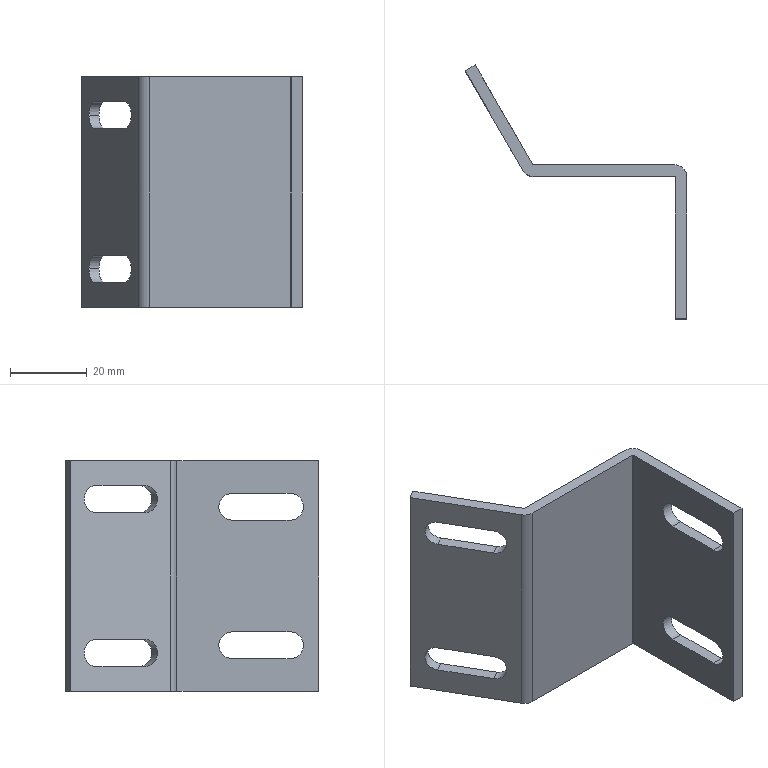Part | STEP file | Z Travel Bracket | 1 solid | 32 faces | box 57.598 x 65.981 x 60 mm | volume 17695 mm3 | plane 18 | cylinder 14 | commonest cylinder face diameters 7 x10 0.2 x2 6.2 x2
STEP:
#1=CARTESIAN_POINT('',(88.934,74.807,53.5));
#2=VERTEX_POINT('',#1);
#3=CARTESIAN_POINT('',(87.184,77.838,50.));
#4=VERTEX_POINT('',#3);
#5=CARTESIAN_POINT('',(88.934,74.807,50.));
#6=DIRECTION('',(-0.866,-0.5,0.));
#7=DIRECTION('',(-0.5,0.866,0.));
#8=AXIS2_PLACEMENT_3D('',#5,#6,#7);
#9=CIRCLE('',#8,3.5);
#10=EDGE_CURVE('',#2,#4,#9,.T.);
#11=ORIENTED_EDGE('',*,*,#10,.T.);
#12=CARTESIAN_POINT('',(89.782,79.338,50.));
#13=VERTEX_POINT('',#12);
#14=CARTESIAN_POINT('',(81.122,74.338,50.));
#15=DIRECTION('',(0.866,0.5,0.));
#16=VECTOR('',#15,1000.);
#17=LINE('',#14,#16);
#18=EDGE_CURVE('',#4,#13,#17,.T.);
#19=ORIENTED_EDGE('',*,*,#18,.T.);
#20=CARTESIAN_POINT('',(91.532,76.307,53.5));
#21=VERTEX_POINT('',#20);
#22=CARTESIAN_POINT('',(91.532,76.307,50.));
#23=DIRECTION('',(-0.866,-0.5,0.));
#24=DIRECTION('',(-0.5,0.866,0.));
#25=AXIS2_PLACEMENT_3D('',#22,#23,#24);
#26=CIRCLE('',#25,3.5);
#27=EDGE_CURVE('',#21,#13,#26,.T.);
#28=ORIENTED_EDGE('',*,*,#27,.F.);
#29=CARTESIAN_POINT('',(82.872,71.307,53.5));
#30=DIRECTION('',(0.866,0.5,0.));
#31=VECTOR('',#30,1000.);
#32=LINE('',#29,#31);
#33=EDGE_CURVE('',#2,#21,#32,.T.);
#34=ORIENTED_EDGE('',*,*,#33,.F.);
#35=EDGE_LOOP('',(#11,#19,#28,#34));
#36=FACE_OUTER_BOUND('',#35,.T.);
#37=CARTESIAN_POINT('',(82.872,71.307,50.));
#38=DIRECTION('',(0.866,0.5,0.));
#39=DIRECTION('',(-0.5,0.866,0.));
#40=AXIS2_PLACEMENT_3D('',#37,#38,#39);
#41=CYLINDRICAL_SURFACE('',#40,3.5);
#42=ADVANCED_FACE('',(#36),#41,.F.);
#43=CARTESIAN_POINT('',(88.934,74.807,13.5));
#44=VERTEX_POINT('',#43);
#45=CARTESIAN_POINT('',(87.184,77.838,10.));
#46=VERTEX_POINT('',#45);
#47=CARTESIAN_POINT('',(88.934,74.807,10.));
#48=DIRECTION('',(-0.866,-0.5,0.));
#49=DIRECTION('',(-0.5,0.866,0.));
#50=AXIS2_PLACEMENT_3D('',#47,#48,#49);
#51=CIRCLE('',#50,3.5);
#52=EDGE_CURVE('',#44,#46,#51,.T.);
#53=ORIENTED_EDGE('',*,*,#52,.T.);
#54=CARTESIAN_POINT('',(89.782,79.338,10.));
#55=VERTEX_POINT('',#54);
#56=CARTESIAN_POINT('',(81.122,74.338,10.));
#57=DIRECTION('',(0.866,0.5,0.));
#58=VECTOR('',#57,1000.);
#59=LINE('',#56,#58);
#60=EDGE_CURVE('',#46,#55,#59,.T.);
#61=ORIENTED_EDGE('',*,*,#60,.T.);
#62=CARTESIAN_POINT('',(91.532,76.307,13.5));
#63=VERTEX_POINT('',#62);
#64=CARTESIAN_POINT('',(91.532,76.307,10.));
#65=DIRECTION('',(-0.866,-0.5,0.));
#66=DIRECTION('',(-0.5,0.866,0.));
#67=AXIS2_PLACEMENT_3D('',#64,#65,#66);
#68=CIRCLE('',#67,3.5);
#69=EDGE_CURVE('',#63,#55,#68,.T.);
#70=ORIENTED_EDGE('',*,*,#69,.F.);
#71=CARTESIAN_POINT('',(82.872,71.307,13.5));
#72=DIRECTION('',(0.866,0.5,0.));
#73=VECTOR('',#72,1000.);
#74=LINE('',#71,#73);
#75=EDGE_CURVE('',#44,#63,#74,.T.);
#76=ORIENTED_EDGE('',*,*,#75,.F.);
#77=EDGE_LOOP('',(#53,#61,#70,#76));
#78=FACE_OUTER_BOUND('',#77,.T.);
#79=CARTESIAN_POINT('',(82.872,71.307,10.));
#80=DIRECTION('',(0.866,0.5,0.));
#81=DIRECTION('',(-0.5,0.866,0.));
#82=AXIS2_PLACEMENT_3D('',#79,#80,#81);
#83=CYLINDRICAL_SURFACE('',#82,3.5);
#84=ADVANCED_FACE('',(#78),#83,.F.);
#85=CARTESIAN_POINT('',(139.682,53.821,60.));
#86=VERTEX_POINT('',#85);
#87=CARTESIAN_POINT('',(139.682,53.821,0.));
#88=VERTEX_POINT('',#87);
#89=CARTESIAN_POINT('',(139.682,53.821,60.));
#90=DIRECTION('',(0.,0.,-1.));
#91=VECTOR('',#90,1000.);
#92=LINE('',#89,#91);
#93=EDGE_CURVE('',#86,#88,#92,.T.);
#94=ORIENTED_EDGE('',*,*,#93,.F.);
#95=CARTESIAN_POINT('',(102.84,53.821,60.));
#96=VERTEX_POINT('',#95);
#97=CARTESIAN_POINT('',(102.782,53.821,60.));
#98=DIRECTION('',(1.,0.,0.));
#99=VECTOR('',#98,1000.);
#100=LINE('',#97,#99);
#101=EDGE_CURVE('',#96,#86,#100,.T.);
#102=ORIENTED_EDGE('',*,*,#101,.F.);
#103=CARTESIAN_POINT('',(102.84,53.821,0.));
#104=VERTEX_POINT('',#103);
#105=CARTESIAN_POINT('',(102.84,53.821,60.));
#106=DIRECTION('',(0.,0.,1.));
#107=VECTOR('',#106,1000.);
#108=LINE('',#105,#107);
#109=EDGE_CURVE('',#104,#96,#108,.T.);
#110=ORIENTED_EDGE('',*,*,#109,.F.);
#111=CARTESIAN_POINT('',(102.782,53.821,0.));
#112=DIRECTION('',(-1.,0.,0.));
#113=VECTOR('',#112,1000.);
#114=LINE('',#111,#113);
#115=EDGE_CURVE('',#88,#104,#114,.T.);
#116=ORIENTED_EDGE('',*,*,#115,.F.);
#117=EDGE_LOOP('',(#94,#102,#110,#116));
#118=FACE_OUTER_BOUND('',#117,.T.);
#119=CARTESIAN_POINT('',(102.782,53.821,60.));
#120=DIRECTION('',(0.,1.,0.));
#121=DIRECTION('',(0.,0.,1.));
#122=AXIS2_PLACEMENT_3D('',#119,#120,#121);
#123=PLANE('',#122);
#124=ADVANCED_FACE('',(#118),#123,.F.);
#125=ORIENTED_EDGE('',*,*,#115,.T.);
#126=CARTESIAN_POINT('',(100.155,55.371,0.));
#127=VERTEX_POINT('',#126);
#128=CARTESIAN_POINT('',(102.84,56.921,0.));
#129=DIRECTION('',(0.,0.,1.));
#130=DIRECTION('',(-1.,0.,0.));
#131=AXIS2_PLACEMENT_3D('',#128,#129,#130);
#132=CIRCLE('',#131,3.1);
#133=EDGE_CURVE('',#127,#104,#132,.T.);
#134=ORIENTED_EDGE('',*,*,#133,.F.);
#135=CARTESIAN_POINT('',(85.184,81.302,0.));
#136=VERTEX_POINT('',#135);
#137=CARTESIAN_POINT('',(85.184,81.302,0.));
#138=DIRECTION('',(-0.5,0.866,0.));
#139=VECTOR('',#138,1000.);
#140=LINE('',#137,#139);
#141=EDGE_CURVE('',#127,#136,#140,.T.);
#142=ORIENTED_EDGE('',*,*,#141,.T.);
#143=CARTESIAN_POINT('',(87.782,82.802,0.));
#144=VERTEX_POINT('',#143);
#145=CARTESIAN_POINT('',(85.184,81.302,0.));
#146=DIRECTION('',(0.866,0.5,0.));
#147=VECTOR('',#146,1000.);
#148=LINE('',#145,#147);
#149=EDGE_CURVE('',#136,#144,#148,.T.);
#150=ORIENTED_EDGE('',*,*,#149,.T.);
#151=CARTESIAN_POINT('',(102.753,56.871,0.));
#152=VERTEX_POINT('',#151);
#153=CARTESIAN_POINT('',(87.782,82.802,0.));
#154=DIRECTION('',(0.5,-0.866,0.));
#155=VECTOR('',#154,1000.);
#156=LINE('',#153,#155);
#157=EDGE_CURVE('',#144,#152,#156,.T.);
#158=ORIENTED_EDGE('',*,*,#157,.T.);
#159=CARTESIAN_POINT('',(102.84,56.821,0.));
#160=VERTEX_POINT('',#159);
#161=CARTESIAN_POINT('',(102.84,56.921,0.));
#162=DIRECTION('',(0.,0.,1.));
#163=DIRECTION('',(-1.,0.,0.));
#164=AXIS2_PLACEMENT_3D('',#161,#162,#163);
#165=CIRCLE('',#164,0.1);
#166=EDGE_CURVE('',#152,#160,#165,.T.);
#167=ORIENTED_EDGE('',*,*,#166,.T.);
#168=CARTESIAN_POINT('',(139.682,56.821,0.));
#169=VERTEX_POINT('',#168);
#170=CARTESIAN_POINT('',(139.782,56.821,0.));
#171=DIRECTION('',(1.,0.,0.));
#172=VECTOR('',#171,1000.);
#173=LINE('',#170,#172);
#174=EDGE_CURVE('',#160,#169,#173,.T.);
#175=ORIENTED_EDGE('',*,*,#174,.T.);
#176=CARTESIAN_POINT('',(142.782,53.721,0.));
#177=VERTEX_POINT('',#176);
#178=CARTESIAN_POINT('',(139.682,53.721,0.));
#179=DIRECTION('',(0.,0.,-1.));
#180=DIRECTION('',(-1.,0.,0.));
#181=AXIS2_PLACEMENT_3D('',#178,#179,#180);
#182=CIRCLE('',#181,3.1);
#183=EDGE_CURVE('',#169,#177,#182,.T.);
#184=ORIENTED_EDGE('',*,*,#183,.T.);
#185=CARTESIAN_POINT('',(142.782,16.821,0.));
#186=VERTEX_POINT('',#185);
#187=CARTESIAN_POINT('',(142.782,53.721,0.));
#188=DIRECTION('',(0.,1.,0.));
#189=VECTOR('',#188,1000.);
#190=LINE('',#187,#189);
#191=EDGE_CURVE('',#186,#177,#190,.T.);
#192=ORIENTED_EDGE('',*,*,#191,.F.);
#193=CARTESIAN_POINT('',(139.782,16.821,0.));
#194=VERTEX_POINT('',#193);
#195=CARTESIAN_POINT('',(139.682,16.821,0.));
#196=DIRECTION('',(1.,0.,0.));
#197=VECTOR('',#196,1000.);
#198=LINE('',#195,#197);
#199=EDGE_CURVE('',#194,#186,#198,.T.);
#200=ORIENTED_EDGE('',*,*,#199,.F.);
#201=CARTESIAN_POINT('',(139.782,53.721,0.));
#202=VERTEX_POINT('',#201);
#203=CARTESIAN_POINT('',(139.782,56.821,0.));
#204=DIRECTION('',(0.,1.,0.));
#205=VECTOR('',#204,1000.);
#206=LINE('',#203,#205);
#207=EDGE_CURVE('',#194,#202,#206,.T.);
#208=ORIENTED_EDGE('',*,*,#207,.T.);
#209=CARTESIAN_POINT('',(139.682,53.721,0.));
#210=DIRECTION('',(0.,0.,1.));
#211=DIRECTION('',(-1.,0.,0.));
#212=AXIS2_PLACEMENT_3D('',#209,#210,#211);
#213=CIRCLE('',#212,0.1);
#214=EDGE_CURVE('',#202,#88,#213,.T.);
#215=ORIENTED_EDGE('',*,*,#214,.T.);
#216=EDGE_LOOP('',(#125,#134,#142,#150,#158,#167,#175,#184,#192,#200,#208,#215));
#217=FACE_OUTER_BOUND('',#216,.T.);
#218=CARTESIAN_POINT('',(139.782,53.721,0.));
#219=DIRECTION('',(0.,0.,-1.));
#220=DIRECTION('',(-1.,0.,0.));
#221=AXIS2_PLACEMENT_3D('',#218,#219,#220);
#222=PLANE('',#221);
#223=ADVANCED_FACE('',(#217),#222,.T.);
#224=CARTESIAN_POINT('',(139.782,53.721,60.));
#225=VERTEX_POINT('',#224);
#226=CARTESIAN_POINT('',(139.782,53.721,60.));
#227=DIRECTION('',(0.,0.,-1.));
#228=VECTOR('',#227,1000.);
#229=LINE('',#226,#228);
#230=EDGE_CURVE('',#225,#202,#229,.T.);
#231=ORIENTED_EDGE('',*,*,#230,.F.);
#232=CARTESIAN_POINT('',(139.682,53.721,60.));
#233=DIRECTION('',(0.,0.,-1.));
#234=DIRECTION('',(-1.,0.,0.));
#235=AXIS2_PLACEMENT_3D('',#232,#233,#234);
#236=CIRCLE('',#235,0.1);
#237=EDGE_CURVE('',#86,#225,#236,.T.);
#238=ORIENTED_EDGE('',*,*,#237,.F.);
#239=ORIENTED_EDGE('',*,*,#93,.T.);
#240=ORIENTED_EDGE('',*,*,#214,.F.);
#241=EDGE_LOOP('',(#231,#238,#239,#240));
#242=FACE_OUTER_BOUND('',#241,.T.);
#243=CARTESIAN_POINT('',(139.682,53.721,60.));
#244=DIRECTION('',(0.,0.,-1.));
#245=DIRECTION('',(-1.,0.,0.));
#246=AXIS2_PLACEMENT_3D('',#243,#244,#245);
#247=CYLINDRICAL_SURFACE('',#246,0.1);
#248=ADVANCED_FACE('',(#242),#247,.F.);
#249=ORIENTED_EDGE('',*,*,#101,.T.);
#250=ORIENTED_EDGE('',*,*,#237,.T.);
#251=CARTESIAN_POINT('',(139.782,16.821,60.));
#252=VERTEX_POINT('',#251);
#253=CARTESIAN_POINT('',(139.782,56.821,60.));
#254=DIRECTION('',(0.,-1.,0.));
#255=VECTOR('',#254,1000.);
#256=LINE('',#253,#255);
#257=EDGE_CURVE('',#225,#252,#256,.T.);
#258=ORIENTED_EDGE('',*,*,#257,.T.);
#259=CARTESIAN_POINT('',(142.782,16.821,60.));
#260=VERTEX_POINT('',#259);
#261=CARTESIAN_POINT('',(142.782,16.821,60.));
#262=DIRECTION('',(-1.,0.,0.));
#263=VECTOR('',#262,1000.);
#264=LINE('',#261,#263);
#265=EDGE_CURVE('',#260,#252,#264,.T.);
#266=ORIENTED_EDGE('',*,*,#265,.F.);
#267=CARTESIAN_POINT('',(142.782,53.721,60.));
#268=VERTEX_POINT('',#267);
#269=CARTESIAN_POINT('',(142.782,53.821,60.));
#270=DIRECTION('',(0.,1.,0.));
#271=VECTOR('',#270,1000.);
#272=LINE('',#269,#271);
#273=EDGE_CURVE('',#260,#268,#272,.T.);
#274=ORIENTED_EDGE('',*,*,#273,.T.);
#275=CARTESIAN_POINT('',(139.682,56.821,60.));
#276=VERTEX_POINT('',#275);
#277=CARTESIAN_POINT('',(139.682,53.721,60.));
#278=DIRECTION('',(0.,0.,1.));
#279=DIRECTION('',(-1.,0.,0.));
#280=AXIS2_PLACEMENT_3D('',#277,#278,#279);
#281=CIRCLE('',#280,3.1);
#282=EDGE_CURVE('',#268,#276,#281,.T.);
#283=ORIENTED_EDGE('',*,*,#282,.T.);
#284=CARTESIAN_POINT('',(102.84,56.821,60.));
#285=VERTEX_POINT('',#284);
#286=CARTESIAN_POINT('',(100.155,56.821,60.));
#287=DIRECTION('',(-1.,0.,0.));
#288=VECTOR('',#287,1000.);
#289=LINE('',#286,#288);
#290=EDGE_CURVE('',#276,#285,#289,.T.);
#291=ORIENTED_EDGE('',*,*,#290,.T.);
#292=CARTESIAN_POINT('',(102.753,56.871,60.));
#293=VERTEX_POINT('',#292);
#294=CARTESIAN_POINT('',(102.84,56.921,60.));
#295=DIRECTION('',(0.,0.,-1.));
#296=DIRECTION('',(-1.,0.,0.));
#297=AXIS2_PLACEMENT_3D('',#294,#295,#296);
#298=CIRCLE('',#297,0.1);
#299=EDGE_CURVE('',#285,#293,#298,.T.);
#300=ORIENTED_EDGE('',*,*,#299,.T.);
#301=CARTESIAN_POINT('',(87.782,82.802,60.));
#302=VERTEX_POINT('',#301);
#303=CARTESIAN_POINT('',(102.753,56.871,60.));
#304=DIRECTION('',(-0.5,0.866,0.));
#305=VECTOR('',#304,1000.);
#306=LINE('',#303,#305);
#307=EDGE_CURVE('',#293,#302,#306,.T.);
#308=ORIENTED_EDGE('',*,*,#307,.T.);
#309=CARTESIAN_POINT('',(85.184,81.302,60.));
#310=VERTEX_POINT('',#309);
#311=CARTESIAN_POINT('',(87.782,82.802,60.));
#312=DIRECTION('',(-0.866,-0.5,0.));
#313=VECTOR('',#312,1000.);
#314=LINE('',#311,#313);
#315=EDGE_CURVE('',#302,#310,#314,.T.);
#316=ORIENTED_EDGE('',*,*,#315,.T.);
#317=CARTESIAN_POINT('',(100.155,55.371,60.));
#318=VERTEX_POINT('',#317);
#319=CARTESIAN_POINT('',(85.184,81.302,60.));
#320=DIRECTION('',(0.5,-0.866,0.));
#321=VECTOR('',#320,1000.);
#322=LINE('',#319,#321);
#323=EDGE_CURVE('',#310,#318,#322,.T.);
#324=ORIENTED_EDGE('',*,*,#323,.T.);
#325=CARTESIAN_POINT('',(102.84,56.921,60.));
#326=DIRECTION('',(0.,0.,-1.));
#327=DIRECTION('',(-1.,0.,0.));
#328=AXIS2_PLACEMENT_3D('',#325,#326,#327);
#329=CIRCLE('',#328,3.1);
#330=EDGE_CURVE('',#96,#318,#329,.T.);
#331=ORIENTED_EDGE('',*,*,#330,.F.);
#332=EDGE_LOOP('',(#249,#250,#258,#266,#274,#283,#291,#300,#308,#316,#324,#331));
#333=FACE_OUTER_BOUND('',#332,.T.);
#334=CARTESIAN_POINT('',(100.155,55.371,60.));
#335=DIRECTION('',(0.,0.,1.));
#336=DIRECTION('',(1.,0.,0.));
#337=AXIS2_PLACEMENT_3D('',#334,#335,#336);
#338=PLANE('',#337);
#339=ADVANCED_FACE('',(#333),#338,.T.);
#340=ORIENTED_EDGE('',*,*,#330,.T.);
#341=CARTESIAN_POINT('',(100.155,55.371,60.));
#342=DIRECTION('',(0.,0.,-1.));
#343=VECTOR('',#342,1000.);
#344=LINE('',#341,#343);
#345=EDGE_CURVE('',#318,#127,#344,.T.);
#346=ORIENTED_EDGE('',*,*,#345,.T.);
#347=ORIENTED_EDGE('',*,*,#133,.T.);
#348=ORIENTED_EDGE('',*,*,#109,.T.);
#349=EDGE_LOOP('',(#340,#346,#347,#348));
#350=FACE_OUTER_BOUND('',#349,.T.);
#351=CARTESIAN_POINT('',(102.84,56.921,60.));
#352=DIRECTION('',(0.,0.,-1.));
#353=DIRECTION('',(-1.,0.,0.));
#354=AXIS2_PLACEMENT_3D('',#351,#352,#353);
#355=CYLINDRICAL_SURFACE('',#354,3.1);
#356=ADVANCED_FACE('',(#350),#355,.T.);
#357=ORIENTED_EDGE('',*,*,#290,.F.);
#358=CARTESIAN_POINT('',(139.682,56.821,60.));
#359=DIRECTION('',(0.,0.,-1.));
#360=VECTOR('',#359,1000.);
#361=LINE('',#358,#360);
#362=EDGE_CURVE('',#276,#169,#361,.T.);
#363=ORIENTED_EDGE('',*,*,#362,.T.);
#364=ORIENTED_EDGE('',*,*,#174,.F.);
#365=CARTESIAN_POINT('',(102.84,56.821,60.));
#366=DIRECTION('',(0.,0.,1.));
#367=VECTOR('',#366,1000.);
#368=LINE('',#365,#367);
#369=EDGE_CURVE('',#160,#285,#368,.T.);
#370=ORIENTED_EDGE('',*,*,#369,.T.);
#371=EDGE_LOOP('',(#357,#363,#364,#370));
#372=FACE_OUTER_BOUND('',#371,.T.);
#373=CARTESIAN_POINT('',(102.782,56.821,60.));
#374=DIRECTION('',(0.,1.,0.));
#375=DIRECTION('',(0.,0.,1.));
#376=AXIS2_PLACEMENT_3D('',#373,#374,#375);
#377=PLANE('',#376);
#378=ADVANCED_FACE('',(#372),#377,.T.);
#379=CARTESIAN_POINT('',(139.782,16.821,60.));
#380=DIRECTION('',(0.,0.,-1.));
#381=VECTOR('',#380,1000.);
#382=LINE('',#379,#381);
#383=EDGE_CURVE('',#252,#194,#382,.T.);
#384=ORIENTED_EDGE('',*,*,#383,.F.);
#385=ORIENTED_EDGE('',*,*,#257,.F.);
#386=ORIENTED_EDGE('',*,*,#230,.T.);
#387=ORIENTED_EDGE('',*,*,#207,.F.);
#388=EDGE_LOOP('',(#384,#385,#386,#387));
#389=FACE_OUTER_BOUND('',#388,.T.);
#390=CARTESIAN_POINT('',(139.782,39.321,51.5));
#391=VERTEX_POINT('',#390);
#392=CARTESIAN_POINT('',(139.782,39.321,44.5));
#393=VERTEX_POINT('',#392);
#394=CARTESIAN_POINT('',(139.782,39.321,48.));
#395=DIRECTION('',(-1.,0.,0.));
#396=DIRECTION('',(0.,0.,-1.));
#397=AXIS2_PLACEMENT_3D('',#394,#395,#396);
#398=CIRCLE('',#397,3.5);
#399=EDGE_CURVE('',#391,#393,#398,.T.);
#400=ORIENTED_EDGE('',*,*,#399,.F.);
#401=CARTESIAN_POINT('',(139.782,24.321,51.5));
#402=VERTEX_POINT('',#401);
#403=CARTESIAN_POINT('',(139.782,56.821,51.5));
#404=DIRECTION('',(0.,1.,0.));
#405=VECTOR('',#404,1000.);
#406=LINE('',#403,#405);
#407=EDGE_CURVE('',#402,#391,#406,.T.);
#408=ORIENTED_EDGE('',*,*,#407,.F.);
#409=CARTESIAN_POINT('',(139.782,24.321,44.5));
#410=VERTEX_POINT('',#409);
#411=CARTESIAN_POINT('',(139.782,24.321,48.));
#412=DIRECTION('',(-1.,0.,0.));
#413=DIRECTION('',(0.,0.,-1.));
#414=AXIS2_PLACEMENT_3D('',#411,#412,#413);
#415=CIRCLE('',#414,3.5);
#416=EDGE_CURVE('',#410,#402,#415,.T.);
#417=ORIENTED_EDGE('',*,*,#416,.F.);
#418=CARTESIAN_POINT('',(139.782,56.821,44.5));
#419=DIRECTION('',(0.,-1.,0.));
#420=VECTOR('',#419,1000.);
#421=LINE('',#418,#420);
#422=EDGE_CURVE('',#393,#410,#421,.T.);
#423=ORIENTED_EDGE('',*,*,#422,.F.);
#424=EDGE_LOOP('',(#400,#408,#417,#423));
#425=FACE_BOUND('',#424,.T.);
#426=CARTESIAN_POINT('',(139.782,39.321,15.5));
#427=VERTEX_POINT('',#426);
#428=CARTESIAN_POINT('',(139.782,39.321,8.5));
#429=VERTEX_POINT('',#428);
#430=CARTESIAN_POINT('',(139.782,39.321,12.));
#431=DIRECTION('',(-1.,0.,0.));
#432=DIRECTION('',(0.,0.,-1.));
#433=AXIS2_PLACEMENT_3D('',#430,#431,#432);
#434=CIRCLE('',#433,3.5);
#435=EDGE_CURVE('',#427,#429,#434,.T.);
#436=ORIENTED_EDGE('',*,*,#435,.F.);
#437=CARTESIAN_POINT('',(139.782,24.321,15.5));
#438=VERTEX_POINT('',#437);
#439=CARTESIAN_POINT('',(139.782,56.821,15.5));
#440=DIRECTION('',(0.,1.,0.));
#441=VECTOR('',#440,1000.);
#442=LINE('',#439,#441);
#443=EDGE_CURVE('',#438,#427,#442,.T.);
#444=ORIENTED_EDGE('',*,*,#443,.F.);
#445=CARTESIAN_POINT('',(139.782,24.321,8.5));
#446=VERTEX_POINT('',#445);
#447=CARTESIAN_POINT('',(139.782,24.321,12.));
#448=DIRECTION('',(-1.,0.,0.));
#449=DIRECTION('',(0.,0.,-1.));
#450=AXIS2_PLACEMENT_3D('',#447,#448,#449);
#451=CIRCLE('',#450,3.5);
#452=EDGE_CURVE('',#446,#438,#451,.T.);
#453=ORIENTED_EDGE('',*,*,#452,.F.);
#454=CARTESIAN_POINT('',(139.782,56.821,8.5));
#455=DIRECTION('',(0.,-1.,0.));
#456=VECTOR('',#455,1000.);
#457=LINE('',#454,#456);
#458=EDGE_CURVE('',#429,#446,#457,.T.);
#459=ORIENTED_EDGE('',*,*,#458,.F.);
#460=EDGE_LOOP('',(#436,#444,#453,#459));
#461=FACE_BOUND('',#460,.T.);
#462=CARTESIAN_POINT('',(139.782,56.821,60.));
#463=DIRECTION('',(1.,0.,0.));
#464=DIRECTION('',(0.,0.,-1.));
#465=AXIS2_PLACEMENT_3D('',#462,#463,#464);
#466=PLANE('',#465);
#467=ADVANCED_FACE('',(#389,#425,#461),#466,.F.);
#468=ORIENTED_EDGE('',*,*,#345,.F.);
#469=ORIENTED_EDGE('',*,*,#323,.F.);
#470=CARTESIAN_POINT('',(85.184,81.302,60.));
#471=DIRECTION('',(0.,0.,1.));
#472=VECTOR('',#471,1000.);
#473=LINE('',#470,#472);
#474=EDGE_CURVE('',#136,#310,#473,.T.);
#475=ORIENTED_EDGE('',*,*,#474,.F.);
#476=ORIENTED_EDGE('',*,*,#141,.F.);
#477=EDGE_LOOP('',(#468,#469,#475,#476));
#478=FACE_OUTER_BOUND('',#477,.T.);
#479=ORIENTED_EDGE('',*,*,#10,.F.);
#480=CARTESIAN_POINT('',(96.434,61.816,53.5));
#481=VERTEX_POINT('',#480);
#482=CARTESIAN_POINT('',(85.184,81.302,53.5));
#483=DIRECTION('',(-0.5,0.866,0.));
#484=VECTOR('',#483,1000.);
#485=LINE('',#482,#484);
#486=EDGE_CURVE('',#481,#2,#485,.T.);
#487=ORIENTED_EDGE('',*,*,#486,.F.);
#488=CARTESIAN_POINT('',(96.434,61.816,46.5));
#489=VERTEX_POINT('',#488);
#490=CARTESIAN_POINT('',(96.434,61.816,50.));
#491=DIRECTION('',(-0.866,-0.5,0.));
#492=DIRECTION('',(-0.5,0.866,0.));
#493=AXIS2_PLACEMENT_3D('',#490,#491,#492);
#494=CIRCLE('',#493,3.5);
#495=EDGE_CURVE('',#489,#481,#494,.T.);
#496=ORIENTED_EDGE('',*,*,#495,.F.);
#497=CARTESIAN_POINT('',(88.934,74.807,46.5));
#498=VERTEX_POINT('',#497);
#499=CARTESIAN_POINT('',(85.184,81.302,46.5));
#500=DIRECTION('',(0.5,-0.866,0.));
#501=VECTOR('',#500,1000.);
#502=LINE('',#499,#501);
#503=EDGE_CURVE('',#498,#489,#502,.T.);
#504=ORIENTED_EDGE('',*,*,#503,.F.);
#505=CARTESIAN_POINT('',(88.934,74.807,50.));
#506=DIRECTION('',(-0.866,-0.5,0.));
#507=DIRECTION('',(-0.5,0.866,0.));
#508=AXIS2_PLACEMENT_3D('',#505,#506,#507);
#509=CIRCLE('',#508,3.5);
#510=EDGE_CURVE('',#4,#498,#509,.T.);
#511=ORIENTED_EDGE('',*,*,#510,.F.);
#512=EDGE_LOOP('',(#479,#487,#496,#504,#511));
#513=FACE_BOUND('',#512,.T.);
#514=ORIENTED_EDGE('',*,*,#52,.F.);
#515=CARTESIAN_POINT('',(96.434,61.816,13.5));
#516=VERTEX_POINT('',#515);
#517=CARTESIAN_POINT('',(85.184,81.302,13.5));
#518=DIRECTION('',(-0.5,0.866,0.));
#519=VECTOR('',#518,1000.);
#520=LINE('',#517,#519);
#521=EDGE_CURVE('',#516,#44,#520,.T.);
#522=ORIENTED_EDGE('',*,*,#521,.F.);
#523=CARTESIAN_POINT('',(96.434,61.816,6.5));
#524=VERTEX_POINT('',#523);
#525=CARTESIAN_POINT('',(96.434,61.816,10.));
#526=DIRECTION('',(-0.866,-0.5,0.));
#527=DIRECTION('',(-0.5,0.866,0.));
#528=AXIS2_PLACEMENT_3D('',#525,#526,#527);
#529=CIRCLE('',#528,3.5);
#530=EDGE_CURVE('',#524,#516,#529,.T.);
#531=ORIENTED_EDGE('',*,*,#530,.F.);
#532=CARTESIAN_POINT('',(88.934,74.807,6.5));
#533=VERTEX_POINT('',#532);
#534=CARTESIAN_POINT('',(85.184,81.302,6.5));
#535=DIRECTION('',(0.5,-0.866,0.));
#536=VECTOR('',#535,1000.);
#537=LINE('',#534,#536);
#538=EDGE_CURVE('',#533,#524,#537,.T.);
#539=ORIENTED_EDGE('',*,*,#538,.F.);
#540=CARTESIAN_POINT('',(88.934,74.807,10.));
#541=DIRECTION('',(-0.866,-0.5,0.));
#542=DIRECTION('',(-0.5,0.866,0.));
#543=AXIS2_PLACEMENT_3D('',#540,#541,#542);
#544=CIRCLE('',#543,3.5);
#545=EDGE_CURVE('',#46,#533,#544,.T.);
#546=ORIENTED_EDGE('',*,*,#545,.F.);
#547=EDGE_LOOP('',(#514,#522,#531,#539,#546));
#548=FACE_BOUND('',#547,.T.);
#549=CARTESIAN_POINT('',(85.184,81.302,60.));
#550=DIRECTION('',(0.866,0.5,0.));
#551=DIRECTION('',(-0.5,0.866,0.));
#552=AXIS2_PLACEMENT_3D('',#549,#550,#551);
#553=PLANE('',#552);
#554=ADVANCED_FACE('',(#478,#513,#548),#553,.F.);
#555=ORIENTED_EDGE('',*,*,#282,.F.);
#556=CARTESIAN_POINT('',(142.782,53.721,60.));
#557=DIRECTION('',(0.,0.,-1.));
#558=VECTOR('',#557,1000.);
#559=LINE('',#556,#558);
#560=EDGE_CURVE('',#268,#177,#559,.T.);
#561=ORIENTED_EDGE('',*,*,#560,.T.);
#562=ORIENTED_EDGE('',*,*,#183,.F.);
#563=ORIENTED_EDGE('',*,*,#362,.F.);
#564=EDGE_LOOP('',(#555,#561,#562,#563));
#565=FACE_OUTER_BOUND('',#564,.T.);
#566=CARTESIAN_POINT('',(139.682,53.721,60.));
#567=DIRECTION('',(0.,0.,-1.));
#568=DIRECTION('',(-1.,0.,0.));
#569=AXIS2_PLACEMENT_3D('',#566,#567,#568);
#570=CYLINDRICAL_SURFACE('',#569,3.1);
#571=ADVANCED_FACE('',(#565),#570,.T.);
#572=CARTESIAN_POINT('',(102.753,56.871,60.));
#573=DIRECTION('',(0.,0.,-1.));
#574=VECTOR('',#573,1000.);
#575=LINE('',#572,#574);
#576=EDGE_CURVE('',#293,#152,#575,.T.);
#577=ORIENTED_EDGE('',*,*,#576,.F.);
#578=ORIENTED_EDGE('',*,*,#299,.F.);
#579=ORIENTED_EDGE('',*,*,#369,.F.);
#580=ORIENTED_EDGE('',*,*,#166,.F.);
#581=EDGE_LOOP('',(#577,#578,#579,#580));
#582=FACE_OUTER_BOUND('',#581,.T.);
#583=CARTESIAN_POINT('',(102.84,56.921,60.));
#584=DIRECTION('',(0.,0.,-1.));
#585=DIRECTION('',(-1.,0.,0.));
#586=AXIS2_PLACEMENT_3D('',#583,#584,#585);
#587=CYLINDRICAL_SURFACE('',#586,0.1);
#588=ADVANCED_FACE('',(#582),#587,.F.);
#589=ORIENTED_EDGE('',*,*,#265,.T.);
#590=ORIENTED_EDGE('',*,*,#383,.T.);
#591=ORIENTED_EDGE('',*,*,#199,.T.);
#592=CARTESIAN_POINT('',(142.782,16.821,60.));
#593=DIRECTION('',(0.,0.,1.));
#594=VECTOR('',#593,1000.);
#595=LINE('',#592,#594);
#596=EDGE_CURVE('',#186,#260,#595,.T.);
#597=ORIENTED_EDGE('',*,*,#596,.T.);
#598=EDGE_LOOP('',(#589,#590,#591,#597));
#599=FACE_OUTER_BOUND('',#598,.T.);
#600=CARTESIAN_POINT('',(142.782,16.821,60.));
#601=DIRECTION('',(0.,-1.,0.));
#602=DIRECTION('',(0.,0.,-1.));
#603=AXIS2_PLACEMENT_3D('',#600,#601,#602);
#604=PLANE('',#603);
#605=ADVANCED_FACE('',(#599),#604,.T.);
#606=CARTESIAN_POINT('',(142.782,39.321,44.5));
#607=VERTEX_POINT('',#606);
#608=CARTESIAN_POINT('',(142.782,24.321,44.5));
#609=VERTEX_POINT('',#608);
#610=CARTESIAN_POINT('',(142.782,39.321,44.5));
#611=DIRECTION('',(0.,-1.,0.));
#612=VECTOR('',#611,1000.);
#613=LINE('',#610,#612);
#614=EDGE_CURVE('',#607,#609,#613,.T.);
#615=ORIENTED_EDGE('',*,*,#614,.F.);
#616=CARTESIAN_POINT('',(132.782,39.321,44.5));
#617=DIRECTION('',(1.,0.,0.));
#618=VECTOR('',#617,1000.);
#619=LINE('',#616,#618);
#620=EDGE_CURVE('',#393,#607,#619,.T.);
#621=ORIENTED_EDGE('',*,*,#620,.F.);
#622=ORIENTED_EDGE('',*,*,#422,.T.);
#623=CARTESIAN_POINT('',(132.782,24.321,44.5));
#624=DIRECTION('',(-1.,0.,0.));
#625=VECTOR('',#624,1000.);
#626=LINE('',#623,#625);
#627=EDGE_CURVE('',#609,#410,#626,.T.);
#628=ORIENTED_EDGE('',*,*,#627,.F.);
#629=EDGE_LOOP('',(#615,#621,#622,#628));
#630=FACE_OUTER_BOUND('',#629,.T.);
#631=CARTESIAN_POINT('',(132.782,39.321,44.5));
#632=DIRECTION('',(0.,0.,-1.));
#633=DIRECTION('',(-1.,0.,0.));
#634=AXIS2_PLACEMENT_3D('',#631,#632,#633);
#635=PLANE('',#634);
#636=ADVANCED_FACE('',(#630),#635,.F.);
#637=CARTESIAN_POINT('',(142.782,39.321,51.5));
#638=VERTEX_POINT('',#637);
#639=CARTESIAN_POINT('',(142.782,39.321,48.));
#640=DIRECTION('',(-1.,0.,0.));
#641=DIRECTION('',(0.,0.,-1.));
#642=AXIS2_PLACEMENT_3D('',#639,#640,#641);
#643=CIRCLE('',#642,3.5);
#644=EDGE_CURVE('',#638,#607,#643,.T.);
#645=ORIENTED_EDGE('',*,*,#644,.F.);
#646=CARTESIAN_POINT('',(132.782,39.321,51.5));
#647=DIRECTION('',(1.,0.,0.));
#648=VECTOR('',#647,1000.);
#649=LINE('',#646,#648);
#650=EDGE_CURVE('',#391,#638,#649,.T.);
#651=ORIENTED_EDGE('',*,*,#650,.F.);
#652=ORIENTED_EDGE('',*,*,#399,.T.);
#653=ORIENTED_EDGE('',*,*,#620,.T.);
#654=EDGE_LOOP('',(#645,#651,#652,#653));
#655=FACE_OUTER_BOUND('',#654,.T.);
#656=CARTESIAN_POINT('',(132.782,39.321,48.));
#657=DIRECTION('',(1.,0.,0.));
#658=DIRECTION('',(0.,0.,-1.));
#659=AXIS2_PLACEMENT_3D('',#656,#657,#658);
#660=CYLINDRICAL_SURFACE('',#659,3.5);
#661=ADVANCED_FACE('',(#655),#660,.F.);
#662=CARTESIAN_POINT('',(142.782,24.321,51.5));
#663=VERTEX_POINT('',#662);
#664=CARTESIAN_POINT('',(142.782,39.321,51.5));
#665=DIRECTION('',(0.,1.,0.));
#666=VECTOR('',#665,1000.);
#667=LINE('',#664,#666);
#668=EDGE_CURVE('',#663,#638,#667,.T.);
#669=ORIENTED_EDGE('',*,*,#668,.F.);
#670=CARTESIAN_POINT('',(132.782,24.321,51.5));
#671=DIRECTION('',(1.,0.,0.));
#672=VECTOR('',#671,1000.);
#673=LINE('',#670,#672);
#674=EDGE_CURVE('',#402,#663,#673,.T.);
#675=ORIENTED_EDGE('',*,*,#674,.F.);
#676=ORIENTED_EDGE('',*,*,#407,.T.);
#677=ORIENTED_EDGE('',*,*,#650,.T.);
#678=EDGE_LOOP('',(#669,#675,#676,#677));
#679=FACE_OUTER_BOUND('',#678,.T.);
#680=CARTESIAN_POINT('',(132.782,39.321,51.5));
#681=DIRECTION('',(0.,0.,1.));
#682=DIRECTION('',(1.,0.,0.));
#683=AXIS2_PLACEMENT_3D('',#680,#681,#682);
#684=PLANE('',#683);
#685=ADVANCED_FACE('',(#679),#684,.F.);
#686=CARTESIAN_POINT('',(142.782,24.321,48.));
#687=DIRECTION('',(-1.,0.,0.));
#688=DIRECTION('',(0.,0.,-1.));
#689=AXIS2_PLACEMENT_3D('',#686,#687,#688);
#690=CIRCLE('',#689,3.5);
#691=EDGE_CURVE('',#609,#663,#690,.T.);
#692=ORIENTED_EDGE('',*,*,#691,.F.);
#693=ORIENTED_EDGE('',*,*,#627,.T.);
#694=ORIENTED_EDGE('',*,*,#416,.T.);
#695=ORIENTED_EDGE('',*,*,#674,.T.);
#696=EDGE_LOOP('',(#692,#693,#694,#695));
#697=FACE_OUTER_BOUND('',#696,.T.);
#698=CARTESIAN_POINT('',(132.782,24.321,48.));
#699=DIRECTION('',(1.,0.,0.));
#700=DIRECTION('',(0.,0.,-1.));
#701=AXIS2_PLACEMENT_3D('',#698,#699,#700);
#702=CYLINDRICAL_SURFACE('',#701,3.5);
#703=ADVANCED_FACE('',(#697),#702,.F.);
#704=CARTESIAN_POINT('',(142.782,39.321,8.5));
#705=VERTEX_POINT('',#704);
#706=CARTESIAN_POINT('',(142.782,24.321,8.5));
#707=VERTEX_POINT('',#706);
#708=CARTESIAN_POINT('',(142.782,39.321,8.5));
#709=DIRECTION('',(0.,-1.,0.));
#710=VECTOR('',#709,1000.);
#711=LINE('',#708,#710);
#712=EDGE_CURVE('',#705,#707,#711,.T.);
#713=ORIENTED_EDGE('',*,*,#712,.F.);
#714=CARTESIAN_POINT('',(132.782,39.321,8.5));
#715=DIRECTION('',(1.,0.,0.));
#716=VECTOR('',#715,1000.);
#717=LINE('',#714,#716);
#718=EDGE_CURVE('',#429,#705,#717,.T.);
#719=ORIENTED_EDGE('',*,*,#718,.F.);
#720=ORIENTED_EDGE('',*,*,#458,.T.);
#721=CARTESIAN_POINT('',(132.782,24.321,8.5));
#722=DIRECTION('',(-1.,0.,0.));
#723=VECTOR('',#722,1000.);
#724=LINE('',#721,#723);
#725=EDGE_CURVE('',#707,#446,#724,.T.);
#726=ORIENTED_EDGE('',*,*,#725,.F.);
#727=EDGE_LOOP('',(#713,#719,#720,#726));
#728=FACE_OUTER_BOUND('',#727,.T.);
#729=CARTESIAN_POINT('',(132.782,39.321,8.5));
#730=DIRECTION('',(0.,0.,-1.));
#731=DIRECTION('',(-1.,0.,0.));
#732=AXIS2_PLACEMENT_3D('',#729,#730,#731);
#733=PLANE('',#732);
#734=ADVANCED_FACE('',(#728),#733,.F.);
#735=CARTESIAN_POINT('',(142.782,39.321,15.5));
#736=VERTEX_POINT('',#735);
#737=CARTESIAN_POINT('',(142.782,39.321,12.));
#738=DIRECTION('',(-1.,0.,0.));
#739=DIRECTION('',(0.,0.,-1.));
#740=AXIS2_PLACEMENT_3D('',#737,#738,#739);
#741=CIRCLE('',#740,3.5);
#742=EDGE_CURVE('',#736,#705,#741,.T.);
#743=ORIENTED_EDGE('',*,*,#742,.F.);
#744=CARTESIAN_POINT('',(132.782,39.321,15.5));
#745=DIRECTION('',(1.,0.,0.));
#746=VECTOR('',#745,1000.);
#747=LINE('',#744,#746);
#748=EDGE_CURVE('',#427,#736,#747,.T.);
#749=ORIENTED_EDGE('',*,*,#748,.F.);
#750=ORIENTED_EDGE('',*,*,#435,.T.);
#751=ORIENTED_EDGE('',*,*,#718,.T.);
#752=EDGE_LOOP('',(#743,#749,#750,#751));
#753=FACE_OUTER_BOUND('',#752,.T.);
#754=CARTESIAN_POINT('',(132.782,39.321,12.));
#755=DIRECTION('',(1.,0.,0.));
#756=DIRECTION('',(0.,0.,-1.));
#757=AXIS2_PLACEMENT_3D('',#754,#755,#756);
#758=CYLINDRICAL_SURFACE('',#757,3.5);
#759=ADVANCED_FACE('',(#753),#758,.F.);
#760=CARTESIAN_POINT('',(142.782,24.321,15.5));
#761=VERTEX_POINT('',#760);
#762=CARTESIAN_POINT('',(142.782,39.321,15.5));
#763=DIRECTION('',(0.,1.,0.));
#764=VECTOR('',#763,1000.);
#765=LINE('',#762,#764);
#766=EDGE_CURVE('',#761,#736,#765,.T.);
#767=ORIENTED_EDGE('',*,*,#766,.F.);
#768=CARTESIAN_POINT('',(132.782,24.321,15.5));
#769=DIRECTION('',(1.,0.,0.));
#770=VECTOR('',#769,1000.);
#771=LINE('',#768,#770);
#772=EDGE_CURVE('',#438,#761,#771,.T.);
#773=ORIENTED_EDGE('',*,*,#772,.F.);
#774=ORIENTED_EDGE('',*,*,#443,.T.);
#775=ORIENTED_EDGE('',*,*,#748,.T.);
#776=EDGE_LOOP('',(#767,#773,#774,#775));
#777=FACE_OUTER_BOUND('',#776,.T.);
#778=CARTESIAN_POINT('',(132.782,39.321,15.5));
#779=DIRECTION('',(0.,0.,1.));
#780=DIRECTION('',(1.,0.,0.));
#781=AXIS2_PLACEMENT_3D('',#778,#779,#780);
#782=PLANE('',#781);
#783=ADVANCED_FACE('',(#777),#782,.F.);
#784=CARTESIAN_POINT('',(142.782,24.321,12.));
#785=DIRECTION('',(-1.,0.,0.));
#786=DIRECTION('',(0.,0.,-1.));
#787=AXIS2_PLACEMENT_3D('',#784,#785,#786);
#788=CIRCLE('',#787,3.5);
#789=EDGE_CURVE('',#707,#761,#788,.T.);
#790=ORIENTED_EDGE('',*,*,#789,.F.);
#791=ORIENTED_EDGE('',*,*,#725,.T.);
#792=ORIENTED_EDGE('',*,*,#452,.T.);
#793=ORIENTED_EDGE('',*,*,#772,.T.);
#794=EDGE_LOOP('',(#790,#791,#792,#793));
#795=FACE_OUTER_BOUND('',#794,.T.);
#796=CARTESIAN_POINT('',(132.782,24.321,12.));
#797=DIRECTION('',(1.,0.,0.));
#798=DIRECTION('',(0.,0.,-1.));
#799=AXIS2_PLACEMENT_3D('',#796,#797,#798);
#800=CYLINDRICAL_SURFACE('',#799,3.5);
#801=ADVANCED_FACE('',(#795),#800,.F.);
#802=ORIENTED_EDGE('',*,*,#315,.F.);
#803=CARTESIAN_POINT('',(87.782,82.802,60.));
#804=DIRECTION('',(0.,0.,-1.));
#805=VECTOR('',#804,1000.);
#806=LINE('',#803,#805);
#807=EDGE_CURVE('',#302,#144,#806,.T.);
#808=ORIENTED_EDGE('',*,*,#807,.T.);
#809=ORIENTED_EDGE('',*,*,#149,.F.);
#810=ORIENTED_EDGE('',*,*,#474,.T.);
#811=EDGE_LOOP('',(#802,#808,#809,#810));
#812=FACE_OUTER_BOUND('',#811,.T.);
#813=CARTESIAN_POINT('',(85.184,81.302,60.));
#814=DIRECTION('',(-0.5,0.866,0.));
#815=DIRECTION('',(-0.866,-0.5,0.));
#816=AXIS2_PLACEMENT_3D('',#813,#814,#815);
#817=PLANE('',#816);
#818=ADVANCED_FACE('',(#812),#817,.T.);
#819=CARTESIAN_POINT('',(91.532,76.307,46.5));
#820=VERTEX_POINT('',#819);
#821=CARTESIAN_POINT('',(99.032,63.316,46.5));
#822=VERTEX_POINT('',#821);
#823=CARTESIAN_POINT('',(91.532,76.307,46.5));
#824=DIRECTION('',(0.5,-0.866,0.));
#825=VECTOR('',#824,1000.);
#826=LINE('',#823,#825);
#827=EDGE_CURVE('',#820,#822,#826,.T.);
#828=ORIENTED_EDGE('',*,*,#827,.F.);
#829=CARTESIAN_POINT('',(88.934,74.807,46.5));
#830=DIRECTION('',(0.866,0.5,0.));
#831=VECTOR('',#830,1000.);
#832=LINE('',#829,#831);
#833=EDGE_CURVE('',#498,#820,#832,.T.);
#834=ORIENTED_EDGE('',*,*,#833,.F.);
#835=ORIENTED_EDGE('',*,*,#503,.T.);
#836=CARTESIAN_POINT('',(99.032,63.316,46.5));
#837=DIRECTION('',(-0.866,-0.5,0.));
#838=VECTOR('',#837,1000.);
#839=LINE('',#836,#838);
#840=EDGE_CURVE('',#822,#489,#839,.T.);
#841=ORIENTED_EDGE('',*,*,#840,.F.);
#842=EDGE_LOOP('',(#828,#834,#835,#841));
#843=FACE_OUTER_BOUND('',#842,.T.);
#844=CARTESIAN_POINT('',(82.872,71.307,46.5));
#845=DIRECTION('',(0.,0.,-1.));
#846=DIRECTION('',(0.,1.,0.));
#847=AXIS2_PLACEMENT_3D('',#844,#845,#846);
#848=PLANE('',#847);
#849=ADVANCED_FACE('',(#843),#848,.F.);
#850=ORIENTED_EDGE('',*,*,#18,.F.);
#851=ORIENTED_EDGE('',*,*,#510,.T.);
#852=ORIENTED_EDGE('',*,*,#833,.T.);
#853=CARTESIAN_POINT('',(91.532,76.307,50.));
#854=DIRECTION('',(-0.866,-0.5,0.));
#855=DIRECTION('',(-0.5,0.866,0.));
#856=AXIS2_PLACEMENT_3D('',#853,#854,#855);
#857=CIRCLE('',#856,3.5);
#858=EDGE_CURVE('',#13,#820,#857,.T.);
#859=ORIENTED_EDGE('',*,*,#858,.F.);
#860=EDGE_LOOP('',(#850,#851,#852,#859));
#861=FACE_OUTER_BOUND('',#860,.T.);
#862=CARTESIAN_POINT('',(82.872,71.307,50.));
#863=DIRECTION('',(0.866,0.5,0.));
#864=DIRECTION('',(-0.5,0.866,0.));
#865=AXIS2_PLACEMENT_3D('',#862,#863,#864);
#866=CYLINDRICAL_SURFACE('',#865,3.5);
#867=ADVANCED_FACE('',(#861),#866,.F.);
#868=CARTESIAN_POINT('',(99.032,63.316,53.5));
#869=VERTEX_POINT('',#868);
#870=CARTESIAN_POINT('',(99.032,63.316,53.5));
#871=DIRECTION('',(-0.5,0.866,0.));
#872=VECTOR('',#871,1000.);
#873=LINE('',#870,#872);
#874=EDGE_CURVE('',#869,#21,#873,.T.);
#875=ORIENTED_EDGE('',*,*,#874,.F.);
#876=CARTESIAN_POINT('',(96.434,61.816,53.5));
#877=DIRECTION('',(0.866,0.5,0.));
#878=VECTOR('',#877,1000.);
#879=LINE('',#876,#878);
#880=EDGE_CURVE('',#481,#869,#879,.T.);
#881=ORIENTED_EDGE('',*,*,#880,.F.);
#882=ORIENTED_EDGE('',*,*,#486,.T.);
#883=ORIENTED_EDGE('',*,*,#33,.T.);
#884=EDGE_LOOP('',(#875,#881,#882,#883));
#885=FACE_OUTER_BOUND('',#884,.T.);
#886=CARTESIAN_POINT('',(82.872,71.307,53.5));
#887=DIRECTION('',(0.,0.,1.));
#888=DIRECTION('',(0.,-1.,0.));
#889=AXIS2_PLACEMENT_3D('',#886,#887,#888);
#890=PLANE('',#889);
#891=ADVANCED_FACE('',(#885),#890,.F.);
#892=CARTESIAN_POINT('',(99.032,63.316,50.));
#893=DIRECTION('',(-0.866,-0.5,0.));
#894=DIRECTION('',(-0.5,0.866,0.));
#895=AXIS2_PLACEMENT_3D('',#892,#893,#894);
#896=CIRCLE('',#895,3.5);
#897=EDGE_CURVE('',#822,#869,#896,.T.);
#898=ORIENTED_EDGE('',*,*,#897,.F.);
#899=ORIENTED_EDGE('',*,*,#840,.T.);
#900=ORIENTED_EDGE('',*,*,#495,.T.);
#901=ORIENTED_EDGE('',*,*,#880,.T.);
#902=EDGE_LOOP('',(#898,#899,#900,#901));
#903=FACE_OUTER_BOUND('',#902,.T.);
#904=CARTESIAN_POINT('',(90.372,58.316,50.));
#905=DIRECTION('',(0.866,0.5,0.));
#906=DIRECTION('',(-0.5,0.866,0.));
#907=AXIS2_PLACEMENT_3D('',#904,#905,#906);
#908=CYLINDRICAL_SURFACE('',#907,3.5);
#909=ADVANCED_FACE('',(#903),#908,.F.);
#910=CARTESIAN_POINT('',(91.532,76.307,6.5));
#911=VERTEX_POINT('',#910);
#912=CARTESIAN_POINT('',(99.032,63.316,6.5));
#913=VERTEX_POINT('',#912);
#914=CARTESIAN_POINT('',(91.532,76.307,6.5));
#915=DIRECTION('',(0.5,-0.866,0.));
#916=VECTOR('',#915,1000.);
#917=LINE('',#914,#916);
#918=EDGE_CURVE('',#911,#913,#917,.T.);
#919=ORIENTED_EDGE('',*,*,#918,.F.);
#920=CARTESIAN_POINT('',(88.934,74.807,6.5));
#921=DIRECTION('',(0.866,0.5,0.));
#922=VECTOR('',#921,1000.);
#923=LINE('',#920,#922);
#924=EDGE_CURVE('',#533,#911,#923,.T.);
#925=ORIENTED_EDGE('',*,*,#924,.F.);
#926=ORIENTED_EDGE('',*,*,#538,.T.);
#927=CARTESIAN_POINT('',(99.032,63.316,6.5));
#928=DIRECTION('',(-0.866,-0.5,0.));
#929=VECTOR('',#928,1000.);
#930=LINE('',#927,#929);
#931=EDGE_CURVE('',#913,#524,#930,.T.);
#932=ORIENTED_EDGE('',*,*,#931,.F.);
#933=EDGE_LOOP('',(#919,#925,#926,#932));
#934=FACE_OUTER_BOUND('',#933,.T.);
#935=CARTESIAN_POINT('',(82.872,71.307,6.5));
#936=DIRECTION('',(0.,0.,-1.));
#937=DIRECTION('',(0.,1.,0.));
#938=AXIS2_PLACEMENT_3D('',#935,#936,#937);
#939=PLANE('',#938);
#940=ADVANCED_FACE('',(#934),#939,.F.);
#941=ORIENTED_EDGE('',*,*,#60,.F.);
#942=ORIENTED_EDGE('',*,*,#545,.T.);
#943=ORIENTED_EDGE('',*,*,#924,.T.);
#944=CARTESIAN_POINT('',(91.532,76.307,10.));
#945=DIRECTION('',(-0.866,-0.5,0.));
#946=DIRECTION('',(-0.5,0.866,0.));
#947=AXIS2_PLACEMENT_3D('',#944,#945,#946);
#948=CIRCLE('',#947,3.5);
#949=EDGE_CURVE('',#55,#911,#948,.T.);
#950=ORIENTED_EDGE('',*,*,#949,.F.);
#951=EDGE_LOOP('',(#941,#942,#943,#950));
#952=FACE_OUTER_BOUND('',#951,.T.);
#953=CARTESIAN_POINT('',(82.872,71.307,10.));
#954=DIRECTION('',(0.866,0.5,0.));
#955=DIRECTION('',(-0.5,0.866,0.));
#956=AXIS2_PLACEMENT_3D('',#953,#954,#955);
#957=CYLINDRICAL_SURFACE('',#956,3.5);
#958=ADVANCED_FACE('',(#952),#957,.F.);
#959=CARTESIAN_POINT('',(99.032,63.316,13.5));
#960=VERTEX_POINT('',#959);
#961=CARTESIAN_POINT('',(99.032,63.316,13.5));
#962=DIRECTION('',(-0.5,0.866,0.));
#963=VECTOR('',#962,1000.);
#964=LINE('',#961,#963);
#965=EDGE_CURVE('',#960,#63,#964,.T.);
#966=ORIENTED_EDGE('',*,*,#965,.F.);
#967=CARTESIAN_POINT('',(96.434,61.816,13.5));
#968=DIRECTION('',(0.866,0.5,0.));
#969=VECTOR('',#968,1000.);
#970=LINE('',#967,#969);
#971=EDGE_CURVE('',#516,#960,#970,.T.);
#972=ORIENTED_EDGE('',*,*,#971,.F.);
#973=ORIENTED_EDGE('',*,*,#521,.T.);
#974=ORIENTED_EDGE('',*,*,#75,.T.);
#975=EDGE_LOOP('',(#966,#972,#973,#974));
#976=FACE_OUTER_BOUND('',#975,.T.);
#977=CARTESIAN_POINT('',(82.872,71.307,13.5));
#978=DIRECTION('',(0.,0.,1.));
#979=DIRECTION('',(0.,-1.,0.));
#980=AXIS2_PLACEMENT_3D('',#977,#978,#979);
#981=PLANE('',#980);
#982=ADVANCED_FACE('',(#976),#981,.F.);
#983=CARTESIAN_POINT('',(99.032,63.316,10.));
#984=DIRECTION('',(-0.866,-0.5,0.));
#985=DIRECTION('',(-0.5,0.866,0.));
#986=AXIS2_PLACEMENT_3D('',#983,#984,#985);
#987=CIRCLE('',#986,3.5);
#988=EDGE_CURVE('',#913,#960,#987,.T.);
#989=ORIENTED_EDGE('',*,*,#988,.F.);
#990=ORIENTED_EDGE('',*,*,#931,.T.);
#991=ORIENTED_EDGE('',*,*,#530,.T.);
#992=ORIENTED_EDGE('',*,*,#971,.T.);
#993=EDGE_LOOP('',(#989,#990,#991,#992));
#994=FACE_OUTER_BOUND('',#993,.T.);
#995=CARTESIAN_POINT('',(90.372,58.316,10.));
#996=DIRECTION('',(0.866,0.5,0.));
#997=DIRECTION('',(-0.5,0.866,0.));
#998=AXIS2_PLACEMENT_3D('',#995,#996,#997);
#999=CYLINDRICAL_SURFACE('',#998,3.5);
#1000=ADVANCED_FACE('',(#994),#999,.F.);
#1001=ORIENTED_EDGE('',*,*,#307,.F.);
#1002=ORIENTED_EDGE('',*,*,#576,.T.);
#1003=ORIENTED_EDGE('',*,*,#157,.F.);
#1004=ORIENTED_EDGE('',*,*,#807,.F.);
#1005=EDGE_LOOP('',(#1001,#1002,#1003,#1004));
#1006=FACE_OUTER_BOUND('',#1005,.T.);
#1007=ORIENTED_EDGE('',*,*,#874,.T.);
#1008=ORIENTED_EDGE('',*,*,#27,.T.);
#1009=ORIENTED_EDGE('',*,*,#858,.T.);
#1010=ORIENTED_EDGE('',*,*,#827,.T.);
#1011=ORIENTED_EDGE('',*,*,#897,.T.);
#1012=EDGE_LOOP('',(#1007,#1008,#1009,#1010,#1011));
#1013=FACE_BOUND('',#1012,.T.);
#1014=ORIENTED_EDGE('',*,*,#965,.T.);
#1015=ORIENTED_EDGE('',*,*,#69,.T.);
#1016=ORIENTED_EDGE('',*,*,#949,.T.);
#1017=ORIENTED_EDGE('',*,*,#918,.T.);
#1018=ORIENTED_EDGE('',*,*,#988,.T.);
#1019=EDGE_LOOP('',(#1014,#1015,#1016,#1017,#1018));
#1020=FACE_BOUND('',#1019,.T.);
#1021=CARTESIAN_POINT('',(87.782,82.802,60.));
#1022=DIRECTION('',(0.866,0.5,0.));
#1023=DIRECTION('',(-0.5,0.866,0.));
#1024=AXIS2_PLACEMENT_3D('',#1021,#1022,#1023);
#1025=PLANE('',#1024);
#1026=ADVANCED_FACE('',(#1006,#1013,#1020),#1025,.T.);
#1027=ORIENTED_EDGE('',*,*,#273,.F.);
#1028=ORIENTED_EDGE('',*,*,#596,.F.);
#1029=ORIENTED_EDGE('',*,*,#191,.T.);
#1030=ORIENTED_EDGE('',*,*,#560,.F.);
#1031=EDGE_LOOP('',(#1027,#1028,#1029,#1030));
#1032=FACE_OUTER_BOUND('',#1031,.T.);
#1033=ORIENTED_EDGE('',*,*,#691,.T.);
#1034=ORIENTED_EDGE('',*,*,#668,.T.);
#1035=ORIENTED_EDGE('',*,*,#644,.T.);
#1036=ORIENTED_EDGE('',*,*,#614,.T.);
#1037=EDGE_LOOP('',(#1033,#1034,#1035,#1036));
#1038=FACE_BOUND('',#1037,.T.);
#1039=ORIENTED_EDGE('',*,*,#789,.T.);
#1040=ORIENTED_EDGE('',*,*,#766,.T.);
#1041=ORIENTED_EDGE('',*,*,#742,.T.);
#1042=ORIENTED_EDGE('',*,*,#712,.T.);
#1043=EDGE_LOOP('',(#1039,#1040,#1041,#1042));
#1044=FACE_BOUND('',#1043,.T.);
#1045=CARTESIAN_POINT('',(142.782,56.821,60.));
#1046=DIRECTION('',(1.,0.,0.));
#1047=DIRECTION('',(0.,0.,-1.));
#1048=AXIS2_PLACEMENT_3D('',#1045,#1046,#1047);
#1049=PLANE('',#1048);
#1050=ADVANCED_FACE('',(#1032,#1038,#1044),#1049,.T.);
#1051=CLOSED_SHELL('',(#42,#84,#124,#223,#248,#339,#356,#378,#467,#554,#571,#588,#605,#636,#661,#685,#703,#734,#759,#783,#801,#818,#849,#867,#891,#909,#940,#958,#982,#1000,#1026,#1050));
#1052=MANIFOLD_SOLID_BREP('',#1051);
#1053=CARTESIAN_POINT('',(0.,0.,0.));
#1054=DIRECTION('',(0.,0.,1.));
#1055=DIRECTION('',(1.,0.,0.));
#1056=AXIS2_PLACEMENT_3D('',#1053,#1054,#1055);
#1057=(LENGTH_UNIT()NAMED_UNIT(*)SI_UNIT(.MILLI.,.METRE.));
#1058=UNCERTAINTY_MEASURE_WITH_UNIT(LENGTH_MEASURE(0.00001),#1057,'','');
#1059=(NAMED_UNIT(*)PLANE_ANGLE_UNIT()SI_UNIT($,.RADIAN.));
#1060=(NAMED_UNIT(*)SI_UNIT($,.STERADIAN.)SOLID_ANGLE_UNIT());
#1061=(GEOMETRIC_REPRESENTATION_CONTEXT(3)GLOBAL_UNCERTAINTY_ASSIGNED_CONTEXT((#1058))GLOBAL_UNIT_ASSIGNED_CONTEXT((#1057,#1059,#1060))REPRESENTATION_CONTEXT('',''));
#1062=ADVANCED_BREP_SHAPE_REPRESENTATION('',(#1052,#1056),#1061);